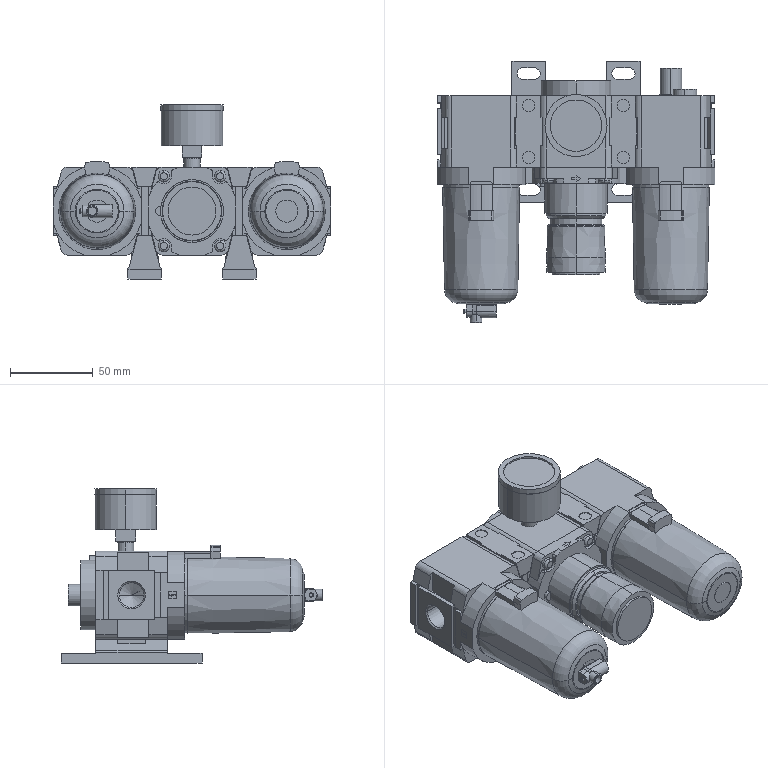Part | SolidWorks | features AEMSimFeature 1 | 15 solids | 979 faces | box 167.4 x 157.9 x 105 mm | volume 781084 mm3 | plane 679 | cylinder 220 | cone 58 | torus 22 | commonest cylinder face diameters 7 x23 8 x21 55 x16 14.95 x12 3 x10 0.6 x9